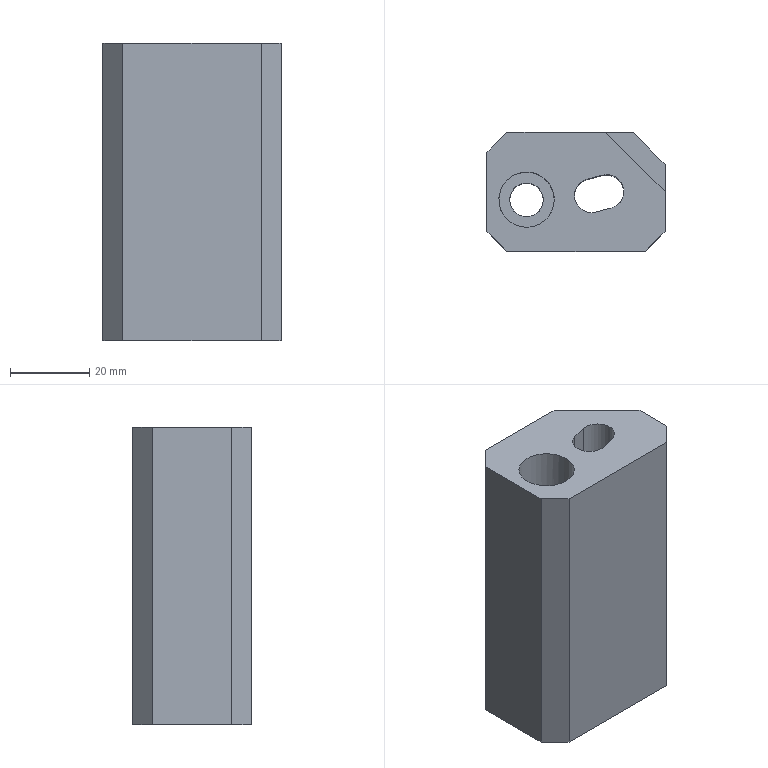Part | STEP file | gslz 2016.10.28-13_id1526_x_t | 1 solid | 19 faces | box 45 x 30 x 75.242 mm | volume 77989 mm3 | plane 15 | cylinder 4 | commonest cylinder face diameters 8.6 x2 8.5 x1 14 x1